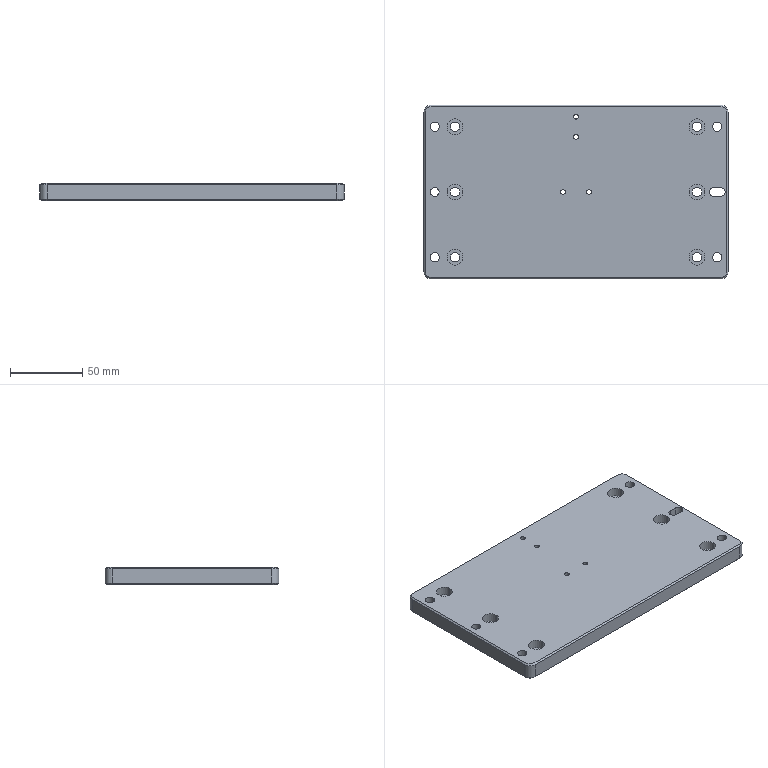Part | STEP file | 03-23 support bracket | 1 solid | 79 faces | box 210 x 120 x 12 mm | volume 293652 mm3 | cylinder 49 | plane 22 | cone 8 | commonest cylinder face diameters 6.6 x12 11 x12 3.3 x8 6.5 x8 6 x5 10 x4